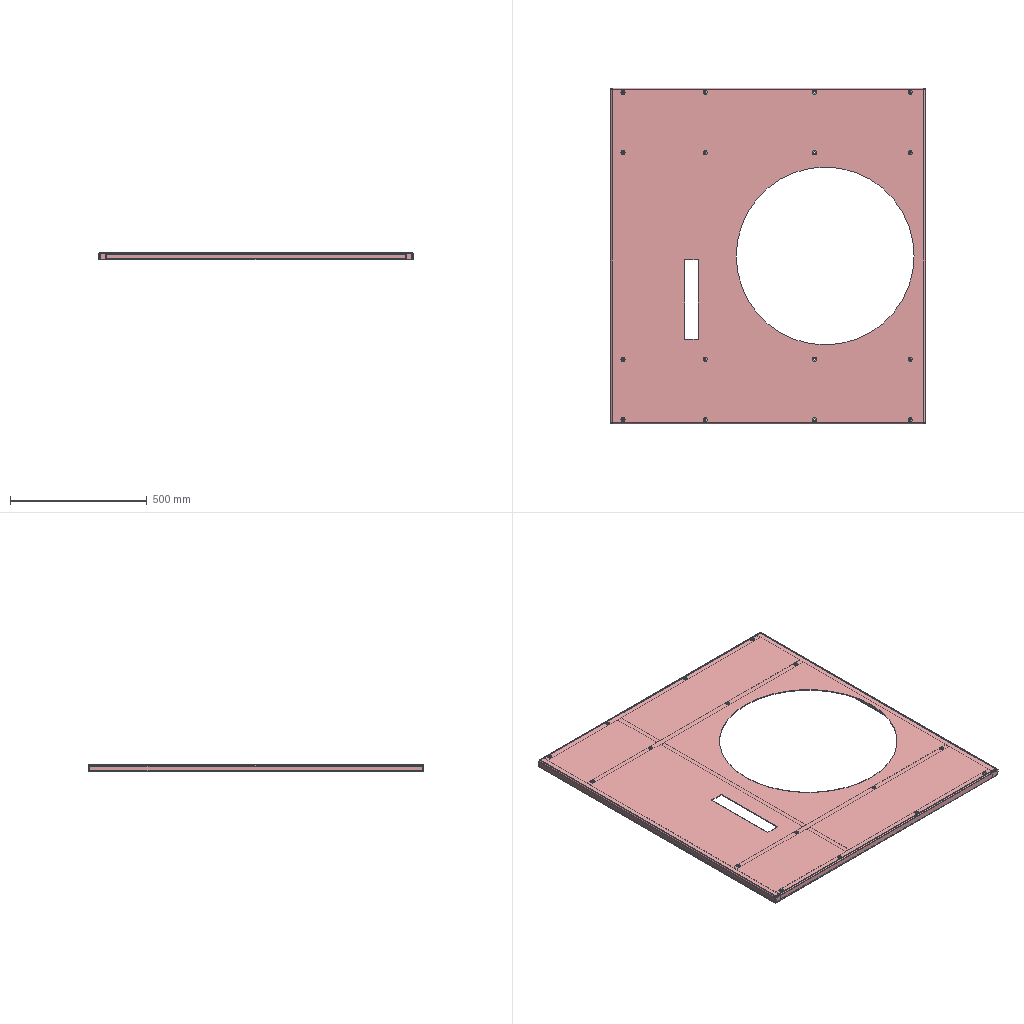Assembly | SolidWorks | 5 different items | 10 placed | box 1150 x 1228 x 28 mm
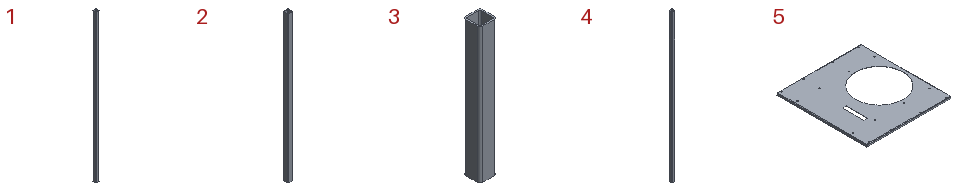Parts list (item | quantity | size | volume | features):
1 | x4 | 25 x 25 x 1094 mm | 190027 mm3 | features Extrusion 1
2 | x1 | 25 x 25 x 730 mm | 126800 mm3 | features Extrusion 1
3 | x2 | 25 x 25 x 198 mm | 34392 mm3 | features Extrusion 1
4 | x2 | 25 x 25 x 1224 mm | 212608 mm3 | features Extrusion 1
5 | x1 | 1150 x 1228 x 28 mm | 3516679 mm3 | features EdgeFlange 3, ICE 2, Extrusion 1, FlatPattern 1, HoleWzd 1, SheetMetal 1, SolidToSheetMetal 1
Mates (type | each side: item.copy, entity, surface, feature):
Coincident | 5.1 face plane | 1.1 face plane
DistanceDim | 1.1 face plane | 1.2 face plane
Coincident | 1.2 face plane | 1.3 face plane
Coincident | 5.1 face plane | 1.3 face plane
Coincident | 5.1 face plane | 2.1 face plane Boss-Extrude1
Coincident | 1.1 face plane | 2.1 face plane Boss-Extrude1
Coincident | 5.1 face plane | 3.1 face plane Boss-Extrude1
Coincident | 2.1 face plane Boss-Extrude1 | 3.1 face plane Boss-Extrude1
Coincident | 1.1 face plane | 3.1 face plane Boss-Extrude1
Coincident | 2.1 face plane Boss-Extrude1 | 3.2 face plane Boss-Extrude1 | 2 times
Coincident | 1.2 face plane | 3.2 face plane Boss-Extrude1
Coincident | 5.1 face plane | 4.1 face plane Boss-Extrude1 | 3 times
Coincident | 5.1 face plane | 4.2 face plane Boss-Extrude1 | 3 times
Coincident | 1.1 face plane | 4.1 face plane Boss-Extrude1
Coincident | 1.3 face plane | 4.1 face plane Boss-Extrude1
DistanceDim | 2.1 face plane Boss-Extrude1 | 4.2 face plane Boss-Extrude1